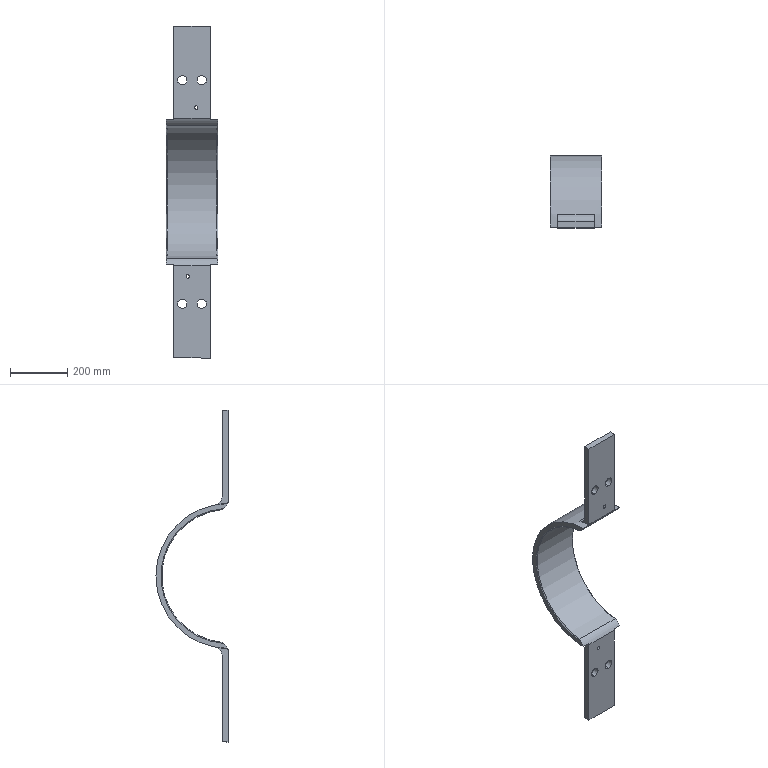Part | SolidWorks | features ICE 4, Fillet 2, MirrorPattern 2, Chamfer 1, Extrusion 1, HoleWzd 1 | 1 solid | 32 faces | box 180 x 251.8 x 1160 mm | volume 4341383 mm3 | cylinder 18 | plane 12 | cone 2 | commonest cylinder face diameters 32 x8 12 x4 60 x2 110 x2 466 x1 506 x1
STEP:
#1=CARTESIAN_POINT('',(-34.,22.,406.));
#2=VERTEX_POINT('',#1);
#3=CARTESIAN_POINT('',(-34.,22.,374.));
#4=VERTEX_POINT('',#3);
#5=CARTESIAN_POINT('',(-34.,22.,390.));
#6=DIRECTION('',(0.,-1.,0.));
#7=DIRECTION('',(0.,0.,-1.));
#8=AXIS2_PLACEMENT_3D('',#5,#6,#7);
#9=CIRCLE('',#8,16.);
#10=EDGE_CURVE('',#2,#4,#9,.T.);
#11=ORIENTED_EDGE('',*,*,#10,.F.);
#12=CARTESIAN_POINT('',(-34.,1.2,406.));
#13=VERTEX_POINT('',#12);
#14=CARTESIAN_POINT('',(-34.,1.2,406.));
#15=DIRECTION('',(0.,-1.,0.));
#16=VECTOR('',#15,1000.);
#17=LINE('',#14,#16);
#18=EDGE_CURVE('',#2,#13,#17,.T.);
#19=ORIENTED_EDGE('',*,*,#18,.T.);
#20=CARTESIAN_POINT('',(-34.,1.2,374.));
#21=VERTEX_POINT('',#20);
#22=CARTESIAN_POINT('',(-34.,1.2,390.));
#23=DIRECTION('',(0.,-1.,0.));
#24=DIRECTION('',(0.,0.,-1.));
#25=AXIS2_PLACEMENT_3D('',#22,#23,#24);
#26=CIRCLE('',#25,16.);
#27=EDGE_CURVE('',#13,#21,#26,.T.);
#28=ORIENTED_EDGE('',*,*,#27,.T.);
#29=CARTESIAN_POINT('',(-34.,1.2,374.));
#30=DIRECTION('',(0.,-1.,0.));
#31=VECTOR('',#30,1000.);
#32=LINE('',#29,#31);
#33=EDGE_CURVE('',#4,#21,#32,.T.);
#34=ORIENTED_EDGE('',*,*,#33,.F.);
#35=EDGE_LOOP('',(#11,#19,#28,#34));
#36=FACE_OUTER_BOUND('',#35,.T.);
#37=CARTESIAN_POINT('',(-34.,1.2,390.));
#38=DIRECTION('',(0.,-1.,0.));
#39=DIRECTION('',(0.,0.,-1.));
#40=AXIS2_PLACEMENT_3D('',#37,#38,#39);
#41=CYLINDRICAL_SURFACE('',#40,16.);
#42=ADVANCED_FACE('',(#36),#41,.F.);
#43=CARTESIAN_POINT('',(34.,22.,406.));
#44=VERTEX_POINT('',#43);
#45=CARTESIAN_POINT('',(34.,22.,374.));
#46=VERTEX_POINT('',#45);
#47=CARTESIAN_POINT('',(34.,22.,390.));
#48=DIRECTION('',(0.,-1.,0.));
#49=DIRECTION('',(0.,0.,-1.));
#50=AXIS2_PLACEMENT_3D('',#47,#48,#49);
#51=CIRCLE('',#50,16.);
#52=EDGE_CURVE('',#44,#46,#51,.T.);
#53=ORIENTED_EDGE('',*,*,#52,.F.);
#54=CARTESIAN_POINT('',(34.,1.2,406.));
#55=VERTEX_POINT('',#54);
#56=CARTESIAN_POINT('',(34.,1.2,406.));
#57=DIRECTION('',(0.,-1.,0.));
#58=VECTOR('',#57,1000.);
#59=LINE('',#56,#58);
#60=EDGE_CURVE('',#44,#55,#59,.T.);
#61=ORIENTED_EDGE('',*,*,#60,.T.);
#62=CARTESIAN_POINT('',(34.,1.2,374.));
#63=VERTEX_POINT('',#62);
#64=CARTESIAN_POINT('',(34.,1.2,390.));
#65=DIRECTION('',(0.,-1.,0.));
#66=DIRECTION('',(0.,0.,-1.));
#67=AXIS2_PLACEMENT_3D('',#64,#65,#66);
#68=CIRCLE('',#67,16.);
#69=EDGE_CURVE('',#55,#63,#68,.T.);
#70=ORIENTED_EDGE('',*,*,#69,.T.);
#71=CARTESIAN_POINT('',(34.,1.2,374.));
#72=DIRECTION('',(0.,-1.,0.));
#73=VECTOR('',#72,1000.);
#74=LINE('',#71,#73);
#75=EDGE_CURVE('',#46,#63,#74,.T.);
#76=ORIENTED_EDGE('',*,*,#75,.F.);
#77=EDGE_LOOP('',(#53,#61,#70,#76));
#78=FACE_OUTER_BOUND('',#77,.T.);
#79=CARTESIAN_POINT('',(34.,1.2,390.));
#80=DIRECTION('',(0.,-1.,0.));
#81=DIRECTION('',(0.,0.,-1.));
#82=AXIS2_PLACEMENT_3D('',#79,#80,#81);
#83=CYLINDRICAL_SURFACE('',#82,16.);
#84=ADVANCED_FACE('',(#78),#83,.F.);
#85=CARTESIAN_POINT('',(34.,22.,-374.));
#86=VERTEX_POINT('',#85);
#87=CARTESIAN_POINT('',(34.,22.,-406.));
#88=VERTEX_POINT('',#87);
#89=CARTESIAN_POINT('',(34.,22.,-390.));
#90=DIRECTION('',(0.,-1.,0.));
#91=DIRECTION('',(0.,0.,-1.));
#92=AXIS2_PLACEMENT_3D('',#89,#90,#91);
#93=CIRCLE('',#92,16.);
#94=EDGE_CURVE('',#86,#88,#93,.T.);
#95=ORIENTED_EDGE('',*,*,#94,.F.);
#96=CARTESIAN_POINT('',(34.,1.2,-374.));
#97=VERTEX_POINT('',#96);
#98=CARTESIAN_POINT('',(34.,1.2,-374.));
#99=DIRECTION('',(0.,-1.,0.));
#100=VECTOR('',#99,1000.);
#101=LINE('',#98,#100);
#102=EDGE_CURVE('',#86,#97,#101,.T.);
#103=ORIENTED_EDGE('',*,*,#102,.T.);
#104=CARTESIAN_POINT('',(34.,1.2,-406.));
#105=VERTEX_POINT('',#104);
#106=CARTESIAN_POINT('',(34.,1.2,-390.));
#107=DIRECTION('',(0.,-1.,0.));
#108=DIRECTION('',(0.,0.,-1.));
#109=AXIS2_PLACEMENT_3D('',#106,#107,#108);
#110=CIRCLE('',#109,16.);
#111=EDGE_CURVE('',#97,#105,#110,.T.);
#112=ORIENTED_EDGE('',*,*,#111,.T.);
#113=CARTESIAN_POINT('',(34.,1.2,-406.));
#114=DIRECTION('',(0.,-1.,0.));
#115=VECTOR('',#114,1000.);
#116=LINE('',#113,#115);
#117=EDGE_CURVE('',#88,#105,#116,.T.);
#118=ORIENTED_EDGE('',*,*,#117,.F.);
#119=EDGE_LOOP('',(#95,#103,#112,#118));
#120=FACE_OUTER_BOUND('',#119,.T.);
#121=CARTESIAN_POINT('',(34.,1.2,-390.));
#122=DIRECTION('',(0.,-1.,0.));
#123=DIRECTION('',(0.,0.,-1.));
#124=AXIS2_PLACEMENT_3D('',#121,#122,#123);
#125=CYLINDRICAL_SURFACE('',#124,16.);
#126=ADVANCED_FACE('',(#120),#125,.F.);
#127=CARTESIAN_POINT('',(-34.,22.,-374.));
#128=VERTEX_POINT('',#127);
#129=CARTESIAN_POINT('',(-34.,22.,-406.));
#130=VERTEX_POINT('',#129);
#131=CARTESIAN_POINT('',(-34.,22.,-390.));
#132=DIRECTION('',(0.,-1.,0.));
#133=DIRECTION('',(0.,0.,-1.));
#134=AXIS2_PLACEMENT_3D('',#131,#132,#133);
#135=CIRCLE('',#134,16.);
#136=EDGE_CURVE('',#128,#130,#135,.T.);
#137=ORIENTED_EDGE('',*,*,#136,.F.);
#138=CARTESIAN_POINT('',(-34.,1.2,-374.));
#139=VERTEX_POINT('',#138);
#140=CARTESIAN_POINT('',(-34.,1.2,-374.));
#141=DIRECTION('',(0.,-1.,0.));
#142=VECTOR('',#141,1000.);
#143=LINE('',#140,#142);
#144=EDGE_CURVE('',#128,#139,#143,.T.);
#145=ORIENTED_EDGE('',*,*,#144,.T.);
#146=CARTESIAN_POINT('',(-34.,1.2,-406.));
#147=VERTEX_POINT('',#146);
#148=CARTESIAN_POINT('',(-34.,1.2,-390.));
#149=DIRECTION('',(0.,-1.,0.));
#150=DIRECTION('',(0.,0.,-1.));
#151=AXIS2_PLACEMENT_3D('',#148,#149,#150);
#152=CIRCLE('',#151,16.);
#153=EDGE_CURVE('',#139,#147,#152,.T.);
#154=ORIENTED_EDGE('',*,*,#153,.T.);
#155=CARTESIAN_POINT('',(-34.,1.2,-406.));
#156=DIRECTION('',(0.,-1.,0.));
#157=VECTOR('',#156,1000.);
#158=LINE('',#155,#157);
#159=EDGE_CURVE('',#130,#147,#158,.T.);
#160=ORIENTED_EDGE('',*,*,#159,.F.);
#161=EDGE_LOOP('',(#137,#145,#154,#160));
#162=FACE_OUTER_BOUND('',#161,.T.);
#163=CARTESIAN_POINT('',(-34.,1.2,-390.));
#164=DIRECTION('',(0.,-1.,0.));
#165=DIRECTION('',(0.,0.,-1.));
#166=AXIS2_PLACEMENT_3D('',#163,#164,#165);
#167=CYLINDRICAL_SURFACE('',#166,16.);
#168=ADVANCED_FACE('',(#162),#167,.F.);
#169=CARTESIAN_POINT('',(-15.,22.,-301.));
#170=VERTEX_POINT('',#169);
#171=CARTESIAN_POINT('',(-15.,22.,-289.));
#172=VERTEX_POINT('',#171);
#173=CARTESIAN_POINT('',(-15.,22.,-295.));
#174=DIRECTION('',(0.,1.,0.));
#175=DIRECTION('',(0.,0.,-1.));
#176=AXIS2_PLACEMENT_3D('',#173,#174,#175);
#177=CIRCLE('',#176,6.);
#178=EDGE_CURVE('',#170,#172,#177,.T.);
#179=ORIENTED_EDGE('',*,*,#178,.T.);
#180=CARTESIAN_POINT('',(-15.,1.2,-289.));
#181=VERTEX_POINT('',#180);
#182=CARTESIAN_POINT('',(-15.,1.2,-289.));
#183=DIRECTION('',(0.,-1.,0.));
#184=VECTOR('',#183,1000.);
#185=LINE('',#182,#184);
#186=EDGE_CURVE('',#172,#181,#185,.T.);
#187=ORIENTED_EDGE('',*,*,#186,.T.);
#188=CARTESIAN_POINT('',(-15.,1.2,-301.));
#189=VERTEX_POINT('',#188);
#190=CARTESIAN_POINT('',(-15.,1.2,-295.));
#191=DIRECTION('',(0.,-1.,0.));
#192=DIRECTION('',(0.,0.,1.));
#193=AXIS2_PLACEMENT_3D('',#190,#191,#192);
#194=CIRCLE('',#193,6.);
#195=EDGE_CURVE('',#181,#189,#194,.T.);
#196=ORIENTED_EDGE('',*,*,#195,.T.);
#197=CARTESIAN_POINT('',(-15.,1.2,-301.));
#198=DIRECTION('',(0.,-1.,0.));
#199=VECTOR('',#198,1000.);
#200=LINE('',#197,#199);
#201=EDGE_CURVE('',#170,#189,#200,.T.);
#202=ORIENTED_EDGE('',*,*,#201,.F.);
#203=EDGE_LOOP('',(#179,#187,#196,#202));
#204=FACE_OUTER_BOUND('',#203,.T.);
#205=CARTESIAN_POINT('',(-15.,1.2,-295.));
#206=DIRECTION('',(0.,-1.,0.));
#207=DIRECTION('',(0.,0.,-1.));
#208=AXIS2_PLACEMENT_3D('',#205,#206,#207);
#209=CYLINDRICAL_SURFACE('',#208,6.);
#210=ADVANCED_FACE('',(#204),#209,.F.);
#211=CARTESIAN_POINT('',(15.,22.,289.));
#212=VERTEX_POINT('',#211);
#213=CARTESIAN_POINT('',(15.,22.,301.));
#214=VERTEX_POINT('',#213);
#215=CARTESIAN_POINT('',(15.,22.,295.));
#216=DIRECTION('',(0.,1.,0.));
#217=DIRECTION('',(0.,0.,-1.));
#218=AXIS2_PLACEMENT_3D('',#215,#216,#217);
#219=CIRCLE('',#218,6.);
#220=EDGE_CURVE('',#212,#214,#219,.T.);
#221=ORIENTED_EDGE('',*,*,#220,.T.);
#222=CARTESIAN_POINT('',(15.,1.2,301.));
#223=VERTEX_POINT('',#222);
#224=CARTESIAN_POINT('',(15.,1.2,301.));
#225=DIRECTION('',(0.,-1.,0.));
#226=VECTOR('',#225,1000.);
#227=LINE('',#224,#226);
#228=EDGE_CURVE('',#214,#223,#227,.T.);
#229=ORIENTED_EDGE('',*,*,#228,.T.);
#230=CARTESIAN_POINT('',(15.,1.2,289.));
#231=VERTEX_POINT('',#230);
#232=CARTESIAN_POINT('',(15.,1.2,295.));
#233=DIRECTION('',(0.,-1.,0.));
#234=DIRECTION('',(0.,0.,1.));
#235=AXIS2_PLACEMENT_3D('',#232,#233,#234);
#236=CIRCLE('',#235,6.);
#237=EDGE_CURVE('',#223,#231,#236,.T.);
#238=ORIENTED_EDGE('',*,*,#237,.T.);
#239=CARTESIAN_POINT('',(15.,1.2,289.));
#240=DIRECTION('',(0.,-1.,0.));
#241=VECTOR('',#240,1000.);
#242=LINE('',#239,#241);
#243=EDGE_CURVE('',#212,#231,#242,.T.);
#244=ORIENTED_EDGE('',*,*,#243,.F.);
#245=EDGE_LOOP('',(#221,#229,#238,#244));
#246=FACE_OUTER_BOUND('',#245,.T.);
#247=CARTESIAN_POINT('',(15.,1.2,295.));
#248=DIRECTION('',(0.,-1.,0.));
#249=DIRECTION('',(0.,0.,-1.));
#250=AXIS2_PLACEMENT_3D('',#247,#248,#249);
#251=CYLINDRICAL_SURFACE('',#250,6.);
#252=ADVANCED_FACE('',(#246),#251,.F.);
#253=CARTESIAN_POINT('',(34.,22.,-390.));
#254=DIRECTION('',(0.,-1.,0.));
#255=DIRECTION('',(0.,0.,-1.));
#256=AXIS2_PLACEMENT_3D('',#253,#254,#255);
#257=CIRCLE('',#256,16.);
#258=EDGE_CURVE('',#88,#86,#257,.T.);
#259=ORIENTED_EDGE('',*,*,#258,.T.);
#260=ORIENTED_EDGE('',*,*,#94,.T.);
#261=EDGE_LOOP('',(#259,#260));
#262=FACE_BOUND('',#261,.T.);
#263=CARTESIAN_POINT('',(-34.,22.,-390.));
#264=DIRECTION('',(0.,-1.,0.));
#265=DIRECTION('',(0.,0.,-1.));
#266=AXIS2_PLACEMENT_3D('',#263,#264,#265);
#267=CIRCLE('',#266,16.);
#268=EDGE_CURVE('',#130,#128,#267,.T.);
#269=ORIENTED_EDGE('',*,*,#268,.T.);
#270=ORIENTED_EDGE('',*,*,#136,.T.);
#271=EDGE_LOOP('',(#269,#270));
#272=FACE_BOUND('',#271,.T.);
#273=CARTESIAN_POINT('',(-63.,22.,-278.182));
#274=VERTEX_POINT('',#273);
#275=CARTESIAN_POINT('',(-63.,22.,-580.));
#276=VERTEX_POINT('',#275);
#277=CARTESIAN_POINT('',(-63.,22.,-252.042));
#278=DIRECTION('',(0.,0.,-1.));
#279=VECTOR('',#278,1000.);
#280=LINE('',#277,#279);
#281=EDGE_CURVE('',#274,#276,#280,.T.);
#282=ORIENTED_EDGE('',*,*,#281,.F.);
#283=CARTESIAN_POINT('',(63.,22.,-278.182));
#284=VERTEX_POINT('',#283);
#285=CARTESIAN_POINT('',(90.,22.,-278.182));
#286=DIRECTION('',(1.,0.,0.));
#287=VECTOR('',#286,1000.);
#288=LINE('',#285,#287);
#289=EDGE_CURVE('',#274,#284,#288,.T.);
#290=ORIENTED_EDGE('',*,*,#289,.T.);
#291=CARTESIAN_POINT('',(63.,22.,-580.));
#292=VERTEX_POINT('',#291);
#293=CARTESIAN_POINT('',(63.,22.,-252.042));
#294=DIRECTION('',(0.,0.,1.));
#295=VECTOR('',#294,1000.);
#296=LINE('',#293,#295);
#297=EDGE_CURVE('',#292,#284,#296,.T.);
#298=ORIENTED_EDGE('',*,*,#297,.F.);
#299=CARTESIAN_POINT('',(90.,22.,-580.));
#300=DIRECTION('',(-1.,0.,0.));
#301=VECTOR('',#300,1000.);
#302=LINE('',#299,#301);
#303=EDGE_CURVE('',#292,#276,#302,.T.);
#304=ORIENTED_EDGE('',*,*,#303,.T.);
#305=EDGE_LOOP('',(#282,#290,#298,#304));
#306=FACE_OUTER_BOUND('',#305,.T.);
#307=ORIENTED_EDGE('',*,*,#178,.F.);
#308=CARTESIAN_POINT('',(-15.,22.,-295.));
#309=DIRECTION('',(0.,1.,0.));
#310=DIRECTION('',(0.,0.,-1.));
#311=AXIS2_PLACEMENT_3D('',#308,#309,#310);
#312=CIRCLE('',#311,6.);
#313=EDGE_CURVE('',#172,#170,#312,.T.);
#314=ORIENTED_EDGE('',*,*,#313,.F.);
#315=EDGE_LOOP('',(#307,#314));
#316=FACE_BOUND('',#315,.T.);
#317=CARTESIAN_POINT('',(90.,22.,-252.042));
#318=DIRECTION('',(0.,-1.,0.));
#319=DIRECTION('',(0.,0.,-1.));
#320=AXIS2_PLACEMENT_3D('',#317,#318,#319);
#321=PLANE('',#320);
#322=ADVANCED_FACE('',(#262,#272,#306,#316),#321,.F.);
#323=CARTESIAN_POINT('',(34.,1.2,-390.));
#324=DIRECTION('',(0.,-1.,0.));
#325=DIRECTION('',(0.,0.,-1.));
#326=AXIS2_PLACEMENT_3D('',#323,#324,#325);
#327=CIRCLE('',#326,16.);
#328=EDGE_CURVE('',#105,#97,#327,.T.);
#329=ORIENTED_EDGE('',*,*,#328,.F.);
#330=ORIENTED_EDGE('',*,*,#111,.F.);
#331=EDGE_LOOP('',(#329,#330));
#332=FACE_BOUND('',#331,.T.);
#333=CARTESIAN_POINT('',(-34.,1.2,-390.));
#334=DIRECTION('',(0.,-1.,0.));
#335=DIRECTION('',(0.,0.,-1.));
#336=AXIS2_PLACEMENT_3D('',#333,#334,#335);
#337=CIRCLE('',#336,16.);
#338=EDGE_CURVE('',#147,#139,#337,.T.);
#339=ORIENTED_EDGE('',*,*,#338,.F.);
#340=ORIENTED_EDGE('',*,*,#153,.F.);
#341=EDGE_LOOP('',(#339,#340));
#342=FACE_BOUND('',#341,.T.);
#343=CARTESIAN_POINT('',(-63.,1.2,-580.));
#344=VERTEX_POINT('',#343);
#345=CARTESIAN_POINT('',(-63.,1.2,-257.102));
#346=VERTEX_POINT('',#345);
#347=CARTESIAN_POINT('',(-63.,1.2,610.));
#348=DIRECTION('',(0.,0.,1.));
#349=VECTOR('',#348,1000.);
#350=LINE('',#347,#349);
#351=EDGE_CURVE('',#344,#346,#350,.T.);
#352=ORIENTED_EDGE('',*,*,#351,.F.);
#353=CARTESIAN_POINT('',(63.,1.2,-580.));
#354=VERTEX_POINT('',#353);
#355=CARTESIAN_POINT('',(90.,1.2,-580.));
#356=DIRECTION('',(-1.,0.,0.));
#357=VECTOR('',#356,1000.);
#358=LINE('',#355,#357);
#359=EDGE_CURVE('',#354,#344,#358,.T.);
#360=ORIENTED_EDGE('',*,*,#359,.F.);
#361=CARTESIAN_POINT('',(63.,1.2,-257.102));
#362=VERTEX_POINT('',#361);
#363=CARTESIAN_POINT('',(63.,1.2,610.));
#364=DIRECTION('',(0.,0.,-1.));
#365=VECTOR('',#364,1000.);
#366=LINE('',#363,#365);
#367=EDGE_CURVE('',#362,#354,#366,.T.);
#368=ORIENTED_EDGE('',*,*,#367,.F.);
#369=CARTESIAN_POINT('',(90.,1.2,-257.102));
#370=DIRECTION('',(-1.,0.,0.));
#371=VECTOR('',#370,1000.);
#372=LINE('',#369,#371);
#373=EDGE_CURVE('',#362,#346,#372,.T.);
#374=ORIENTED_EDGE('',*,*,#373,.T.);
#375=EDGE_LOOP('',(#352,#360,#368,#374));
#376=FACE_OUTER_BOUND('',#375,.T.);
#377=CARTESIAN_POINT('',(-15.,1.2,-295.));
#378=DIRECTION('',(0.,-1.,0.));
#379=DIRECTION('',(0.,0.,1.));
#380=AXIS2_PLACEMENT_3D('',#377,#378,#379);
#381=CIRCLE('',#380,6.);
#382=EDGE_CURVE('',#189,#181,#381,.T.);
#383=ORIENTED_EDGE('',*,*,#382,.F.);
#384=ORIENTED_EDGE('',*,*,#195,.F.);
#385=EDGE_LOOP('',(#383,#384));
#386=FACE_BOUND('',#385,.T.);
#387=CARTESIAN_POINT('',(-90.,1.2,610.));
#388=DIRECTION('',(0.,1.,0.));
#389=DIRECTION('',(0.,0.,1.));
#390=AXIS2_PLACEMENT_3D('',#387,#388,#389);
#391=PLANE('',#390);
#392=ADVANCED_FACE('',(#332,#342,#376,#386),#391,.F.);
#393=CARTESIAN_POINT('',(-34.,22.,390.));
#394=DIRECTION('',(0.,-1.,0.));
#395=DIRECTION('',(0.,0.,-1.));
#396=AXIS2_PLACEMENT_3D('',#393,#394,#395);
#397=CIRCLE('',#396,16.);
#398=EDGE_CURVE('',#4,#2,#397,.T.);
#399=ORIENTED_EDGE('',*,*,#398,.T.);
#400=ORIENTED_EDGE('',*,*,#10,.T.);
#401=EDGE_LOOP('',(#399,#400));
#402=FACE_BOUND('',#401,.T.);
#403=CARTESIAN_POINT('',(34.,22.,390.));
#404=DIRECTION('',(0.,-1.,0.));
#405=DIRECTION('',(0.,0.,-1.));
#406=AXIS2_PLACEMENT_3D('',#403,#404,#405);
#407=CIRCLE('',#406,16.);
#408=EDGE_CURVE('',#46,#44,#407,.T.);
#409=ORIENTED_EDGE('',*,*,#408,.T.);
#410=ORIENTED_EDGE('',*,*,#52,.T.);
#411=EDGE_LOOP('',(#409,#410));
#412=FACE_BOUND('',#411,.T.);
#413=CARTESIAN_POINT('',(-63.,22.,580.));
#414=VERTEX_POINT('',#413);
#415=CARTESIAN_POINT('',(-63.,22.,278.182));
#416=VERTEX_POINT('',#415);
#417=CARTESIAN_POINT('',(-63.,22.,580.));
#418=DIRECTION('',(0.,0.,-1.));
#419=VECTOR('',#418,1000.);
#420=LINE('',#417,#419);
#421=EDGE_CURVE('',#414,#416,#420,.T.);
#422=ORIENTED_EDGE('',*,*,#421,.F.);
#423=CARTESIAN_POINT('',(63.,22.,580.));
#424=VERTEX_POINT('',#423);
#425=CARTESIAN_POINT('',(90.,22.,580.));
#426=DIRECTION('',(-1.,0.,0.));
#427=VECTOR('',#426,1000.);
#428=LINE('',#425,#427);
#429=EDGE_CURVE('',#424,#414,#428,.T.);
#430=ORIENTED_EDGE('',*,*,#429,.F.);
#431=CARTESIAN_POINT('',(63.,22.,278.182));
#432=VERTEX_POINT('',#431);
#433=CARTESIAN_POINT('',(63.,22.,580.));
#434=DIRECTION('',(0.,0.,1.));
#435=VECTOR('',#434,1000.);
#436=LINE('',#433,#435);
#437=EDGE_CURVE('',#432,#424,#436,.T.);
#438=ORIENTED_EDGE('',*,*,#437,.F.);
#439=CARTESIAN_POINT('',(-90.,22.,278.182));
#440=DIRECTION('',(-1.,0.,0.));
#441=VECTOR('',#440,1000.);
#442=LINE('',#439,#441);
#443=EDGE_CURVE('',#432,#416,#442,.T.);
#444=ORIENTED_EDGE('',*,*,#443,.T.);
#445=EDGE_LOOP('',(#422,#430,#438,#444));
#446=FACE_OUTER_BOUND('',#445,.T.);
#447=ORIENTED_EDGE('',*,*,#220,.F.);
#448=CARTESIAN_POINT('',(15.,22.,295.));
#449=DIRECTION('',(0.,1.,0.));
#450=DIRECTION('',(0.,0.,-1.));
#451=AXIS2_PLACEMENT_3D('',#448,#449,#450);
#452=CIRCLE('',#451,6.);
#453=EDGE_CURVE('',#214,#212,#452,.T.);
#454=ORIENTED_EDGE('',*,*,#453,.F.);
#455=EDGE_LOOP('',(#447,#454));
#456=FACE_BOUND('',#455,.T.);
#457=CARTESIAN_POINT('',(90.,22.,580.));
#458=DIRECTION('',(0.,-1.,0.));
#459=DIRECTION('',(0.,0.,-1.));
#460=AXIS2_PLACEMENT_3D('',#457,#458,#459);
#461=PLANE('',#460);
#462=ADVANCED_FACE('',(#402,#412,#446,#456),#461,.F.);
#463=CARTESIAN_POINT('',(-34.,1.2,390.));
#464=DIRECTION('',(0.,-1.,0.));
#465=DIRECTION('',(0.,0.,-1.));
#466=AXIS2_PLACEMENT_3D('',#463,#464,#465);
#467=CIRCLE('',#466,16.);
#468=EDGE_CURVE('',#21,#13,#467,.T.);
#469=ORIENTED_EDGE('',*,*,#468,.F.);
#470=ORIENTED_EDGE('',*,*,#27,.F.);
#471=EDGE_LOOP('',(#469,#470));
#472=FACE_BOUND('',#471,.T.);
#473=CARTESIAN_POINT('',(34.,1.2,390.));
#474=DIRECTION('',(0.,-1.,0.));
#475=DIRECTION('',(0.,0.,-1.));
#476=AXIS2_PLACEMENT_3D('',#473,#474,#475);
#477=CIRCLE('',#476,16.);
#478=EDGE_CURVE('',#63,#55,#477,.T.);
#479=ORIENTED_EDGE('',*,*,#478,.F.);
#480=ORIENTED_EDGE('',*,*,#69,.F.);
#481=EDGE_LOOP('',(#479,#480));
#482=FACE_BOUND('',#481,.T.);
#483=CARTESIAN_POINT('',(-63.,1.2,257.102));
#484=VERTEX_POINT('',#483);
#485=CARTESIAN_POINT('',(-63.,1.2,580.));
#486=VERTEX_POINT('',#485);
#487=CARTESIAN_POINT('',(-63.,1.2,610.));
#488=DIRECTION('',(0.,0.,1.));
#489=VECTOR('',#488,1000.);
#490=LINE('',#487,#489);
#491=EDGE_CURVE('',#484,#486,#490,.T.);
#492=ORIENTED_EDGE('',*,*,#491,.F.);
#493=CARTESIAN_POINT('',(63.,1.2,257.102));
#494=VERTEX_POINT('',#493);
#495=CARTESIAN_POINT('',(90.,1.2,257.102));
#496=DIRECTION('',(1.,0.,0.));
#497=VECTOR('',#496,1000.);
#498=LINE('',#495,#497);
#499=EDGE_CURVE('',#484,#494,#498,.T.);
#500=ORIENTED_EDGE('',*,*,#499,.T.);
#501=CARTESIAN_POINT('',(63.,1.2,580.));
#502=VERTEX_POINT('',#501);
#503=CARTESIAN_POINT('',(63.,1.2,610.));
#504=DIRECTION('',(0.,0.,-1.));
#505=VECTOR('',#504,1000.);
#506=LINE('',#503,#505);
#507=EDGE_CURVE('',#502,#494,#506,.T.);
#508=ORIENTED_EDGE('',*,*,#507,.F.);
#509=CARTESIAN_POINT('',(90.,1.2,580.));
#510=DIRECTION('',(1.,0.,0.));
#511=VECTOR('',#510,1000.);
#512=LINE('',#509,#511);
#513=EDGE_CURVE('',#486,#502,#512,.T.);
#514=ORIENTED_EDGE('',*,*,#513,.F.);
#515=EDGE_LOOP('',(#492,#500,#508,#514));
#516=FACE_OUTER_BOUND('',#515,.T.);
#517=CARTESIAN_POINT('',(15.,1.2,295.));
#518=DIRECTION('',(0.,-1.,0.));
#519=DIRECTION('',(0.,0.,1.));
#520=AXIS2_PLACEMENT_3D('',#517,#518,#519);
#521=CIRCLE('',#520,6.);
#522=EDGE_CURVE('',#231,#223,#521,.T.);
#523=ORIENTED_EDGE('',*,*,#522,.F.);
#524=ORIENTED_EDGE('',*,*,#237,.F.);
#525=EDGE_LOOP('',(#523,#524));
#526=FACE_BOUND('',#525,.T.);
#527=CARTESIAN_POINT('',(-90.,1.2,610.));
#528=DIRECTION('',(0.,1.,0.));
#529=DIRECTION('',(0.,0.,1.));
#530=AXIS2_PLACEMENT_3D('',#527,#528,#529);
#531=PLANE('',#530);
#532=ADVANCED_FACE('',(#472,#482,#516,#526),#531,.F.);
#533=CARTESIAN_POINT('',(-63.,22.,-580.));
#534=DIRECTION('',(0.,-1.,0.));
#535=VECTOR('',#534,1000.);
#536=LINE('',#533,#535);
#537=EDGE_CURVE('',#276,#344,#536,.T.);
#538=ORIENTED_EDGE('',*,*,#537,.F.);
#539=ORIENTED_EDGE('',*,*,#303,.F.);
#540=CARTESIAN_POINT('',(63.,22.,-580.));
#541=DIRECTION('',(0.,1.,0.));
#542=VECTOR('',#541,1000.);
#543=LINE('',#540,#542);
#544=EDGE_CURVE('',#354,#292,#543,.T.);
#545=ORIENTED_EDGE('',*,*,#544,.F.);
#546=ORIENTED_EDGE('',*,*,#359,.T.);
#547=EDGE_LOOP('',(#538,#539,#545,#546));
#548=FACE_OUTER_BOUND('',#547,.T.);
#549=CARTESIAN_POINT('',(90.,22.,-580.));
#550=DIRECTION('',(0.,0.,1.));
#551=DIRECTION('',(1.,0.,0.));
#552=AXIS2_PLACEMENT_3D('',#549,#550,#551);
#553=PLANE('',#552);
#554=ADVANCED_FACE('',(#548),#553,.F.);
#555=CARTESIAN_POINT('',(-63.,46.488,-248.692));
#556=VERTEX_POINT('',#555);
#557=CARTESIAN_POINT('',(-63.,52.,-278.182));
#558=DIRECTION('',(1.,0.,0.));
#559=DIRECTION('',(0.,0.,1.));
#560=AXIS2_PLACEMENT_3D('',#557,#558,#559);
#561=CIRCLE('',#560,30.);
#562=EDGE_CURVE('',#556,#274,#561,.T.);
#563=ORIENTED_EDGE('',*,*,#562,.F.);
#564=CARTESIAN_POINT('',(63.,46.488,-248.692));
#565=VERTEX_POINT('',#564);
#566=CARTESIAN_POINT('',(90.,46.488,-248.692));
#567=DIRECTION('',(-1.,0.,0.));
#568=VECTOR('',#567,1000.);
#569=LINE('',#566,#568);
#570=EDGE_CURVE('',#565,#556,#569,.T.);
#571=ORIENTED_EDGE('',*,*,#570,.F.);
#572=CARTESIAN_POINT('',(63.,52.,-278.182));
#573=DIRECTION('',(-1.,0.,0.));
#574=DIRECTION('',(0.,0.,-1.));
#575=AXIS2_PLACEMENT_3D('',#572,#573,#574);
#576=CIRCLE('',#575,30.);
#577=EDGE_CURVE('',#284,#565,#576,.T.);
#578=ORIENTED_EDGE('',*,*,#577,.F.);
#579=ORIENTED_EDGE('',*,*,#289,.F.);
#580=EDGE_LOOP('',(#563,#571,#578,#579));
#581=FACE_OUTER_BOUND('',#580,.T.);
#582=CARTESIAN_POINT('',(90.,52.,-278.182));
#583=DIRECTION('',(-1.,0.,0.));
#584=DIRECTION('',(0.,0.,1.));
#585=AXIS2_PLACEMENT_3D('',#582,#583,#584);
#586=CYLINDRICAL_SURFACE('',#585,30.);
#587=ADVANCED_FACE('',(#581),#586,.F.);
#588=CARTESIAN_POINT('',(-63.,22.,580.));
#589=DIRECTION('',(0.,1.,0.));
#590=VECTOR('',#589,1000.);
#591=LINE('',#588,#590);
#592=EDGE_CURVE('',#486,#414,#591,.T.);
#593=ORIENTED_EDGE('',*,*,#592,.F.);
#594=ORIENTED_EDGE('',*,*,#513,.T.);
#595=CARTESIAN_POINT('',(63.,22.,580.));
#596=DIRECTION('',(0.,-1.,0.));
#597=VECTOR('',#596,1000.);
#598=LINE('',#595,#597);
#599=EDGE_CURVE('',#424,#502,#598,.T.);
#600=ORIENTED_EDGE('',*,*,#599,.F.);
#601=ORIENTED_EDGE('',*,*,#429,.T.);
#602=EDGE_LOOP('',(#593,#594,#600,#601));
#603=FACE_OUTER_BOUND('',#602,.T.);
#604=CARTESIAN_POINT('',(90.,22.,580.));
#605=DIRECTION('',(0.,0.,-1.));
#606=DIRECTION('',(-1.,0.,0.));
#607=AXIS2_PLACEMENT_3D('',#604,#605,#606);
#608=PLANE('',#607);
#609=ADVANCED_FACE('',(#603),#608,.F.);
#610=CARTESIAN_POINT('',(-63.,46.488,248.692));
#611=VERTEX_POINT('',#610);
#612=CARTESIAN_POINT('',(-63.,52.,278.182));
#613=DIRECTION('',(1.,0.,0.));
#614=DIRECTION('',(0.,0.,1.));
#615=AXIS2_PLACEMENT_3D('',#612,#613,#614);
#616=CIRCLE('',#615,30.);
#617=EDGE_CURVE('',#416,#611,#616,.T.);
#618=ORIENTED_EDGE('',*,*,#617,.F.);
#619=ORIENTED_EDGE('',*,*,#443,.F.);
#620=CARTESIAN_POINT('',(63.,46.488,248.692));
#621=VERTEX_POINT('',#620);
#622=CARTESIAN_POINT('',(63.,52.,278.182));
#623=DIRECTION('',(-1.,0.,0.));
#624=DIRECTION('',(0.,0.,-1.));
#625=AXIS2_PLACEMENT_3D('',#622,#623,#624);
#626=CIRCLE('',#625,30.);
#627=EDGE_CURVE('',#621,#432,#626,.T.);
#628=ORIENTED_EDGE('',*,*,#627,.F.);
#629=CARTESIAN_POINT('',(90.,46.488,248.692));
#630=DIRECTION('',(1.,0.,0.));
#631=VECTOR('',#630,1000.);
#632=LINE('',#629,#631);
#633=EDGE_CURVE('',#611,#621,#632,.T.);
#634=ORIENTED_EDGE('',*,*,#633,.F.);
#635=EDGE_LOOP('',(#618,#619,#628,#634));
#636=FACE_OUTER_BOUND('',#635,.T.);
#637=CARTESIAN_POINT('',(90.,52.,278.182));
#638=DIRECTION('',(-1.,0.,0.));
#639=DIRECTION('',(0.,0.,1.));
#640=AXIS2_PLACEMENT_3D('',#637,#638,#639);
#641=CYLINDRICAL_SURFACE('',#640,30.);
#642=ADVANCED_FACE('',(#636),#641,.F.);
#643=CARTESIAN_POINT('',(-90.,3.113,-252.981));
#644=VERTEX_POINT('',#643);
#645=CARTESIAN_POINT('',(-90.,17.496,-235.351));
#646=VERTEX_POINT('',#645);
#647=CARTESIAN_POINT('',(-90.,52.,-278.182));
#648=DIRECTION('',(-1.,0.,0.));
#649=DIRECTION('',(0.,0.,-1.));
#650=AXIS2_PLACEMENT_3D('',#647,#648,#649);
#651=CIRCLE('',#650,55.);
#652=EDGE_CURVE('',#644,#646,#651,.T.);
#653=ORIENTED_EDGE('',*,*,#652,.T.);
#654=CARTESIAN_POINT('',(-90.,17.496,235.351));
#655=VERTEX_POINT('',#654);
#656=CARTESIAN_POINT('',(-90.,0.,0.));
#657=DIRECTION('',(1.,0.,0.));
#658=DIRECTION('',(0.,0.,-1.));
#659=AXIS2_PLACEMENT_3D('',#656,#657,#658);
#660=CIRCLE('',#659,236.);
#661=EDGE_CURVE('',#646,#655,#660,.T.);
#662=ORIENTED_EDGE('',*,*,#661,.T.);
#663=CARTESIAN_POINT('',(-90.,3.113,252.981));
#664=VERTEX_POINT('',#663);
#665=CARTESIAN_POINT('',(-90.,52.,278.182));
#666=DIRECTION('',(-1.,0.,0.));
#667=DIRECTION('',(0.,0.,-1.));
#668=AXIS2_PLACEMENT_3D('',#665,#666,#667);
#669=CIRCLE('',#668,55.);
#670=EDGE_CURVE('',#655,#664,#669,.T.);
#671=ORIENTED_EDGE('',*,*,#670,.T.);
#672=CARTESIAN_POINT('',(-90.,0.,0.));
#673=DIRECTION('',(1.,0.,0.));
#674=DIRECTION('',(0.,0.,-1.));
#675=AXIS2_PLACEMENT_3D('',#672,#673,#674);
#676=CIRCLE('',#675,253.);
#677=EDGE_CURVE('',#644,#664,#676,.T.);
#678=ORIENTED_EDGE('',*,*,#677,.F.);
#679=EDGE_LOOP('',(#653,#662,#671,#678));
#680=FACE_OUTER_BOUND('',#679,.T.);
#681=CARTESIAN_POINT('',(-90.,0.,0.));
#682=DIRECTION('',(1.,0.,0.));
#683=DIRECTION('',(0.,0.,-1.));
#684=AXIS2_PLACEMENT_3D('',#681,#682,#683);
#685=PLANE('',#684);
#686=ADVANCED_FACE('',(#680),#685,.F.);
#687=CARTESIAN_POINT('',(87.,22.226,231.937));
#688=VERTEX_POINT('',#687);
#689=CARTESIAN_POINT('',(-87.,22.226,231.937));
#690=VERTEX_POINT('',#689);
#691=CARTESIAN_POINT('',(0.,22.226,231.937));
#692=DIRECTION('',(-1.,0.,0.));
#693=VECTOR('',#692,1000.);
#694=LINE('',#691,#693);
#695=EDGE_CURVE('',#688,#690,#694,.T.);
#696=ORIENTED_EDGE('',*,*,#695,.F.);
#697=CARTESIAN_POINT('',(90.,17.496,235.351));
#698=VERTEX_POINT('',#697);
#699=CARTESIAN_POINT('',(87.,22.226,231.937));
#700=CARTESIAN_POINT('',(87.913,20.552,233.016));
#701=CARTESIAN_POINT('',(88.918,18.98,234.156));
#702=CARTESIAN_POINT('',(90.,17.496,235.351));
#703=B_SPLINE_CURVE_WITH_KNOTS('',3,(#699,#700,#701,#702),.UNSPECIFIED.,.F.,.F.,(4,4),(0.,0.006559),.UNSPECIFIED.);
#704=EDGE_CURVE('',#688,#698,#703,.T.);
#705=ORIENTED_EDGE('',*,*,#704,.T.);
#706=CARTESIAN_POINT('',(90.,3.113,252.981));
#707=VERTEX_POINT('',#706);
#708=CARTESIAN_POINT('',(90.,52.,278.182));
#709=DIRECTION('',(1.,0.,0.));
#710=DIRECTION('',(0.,0.,-1.));
#711=AXIS2_PLACEMENT_3D('',#708,#709,#710);
#712=CIRCLE('',#711,55.);
#713=EDGE_CURVE('',#707,#698,#712,.T.);
#714=ORIENTED_EDGE('',*,*,#713,.F.);
#715=CARTESIAN_POINT('',(63.,3.113,252.981));
#716=VERTEX_POINT('',#715);
#717=CARTESIAN_POINT('',(76.5,3.113,252.981));
#718=DIRECTION('',(1.,0.,0.));
#719=VECTOR('',#718,1000.);
#720=LINE('',#717,#719);
#721=EDGE_CURVE('',#716,#707,#720,.T.);
#722=ORIENTED_EDGE('',*,*,#721,.F.);
#723=CARTESIAN_POINT('',(63.,52.,278.182));
#724=DIRECTION('',(-1.,0.,0.));
#725=DIRECTION('',(0.,0.,-1.));
#726=AXIS2_PLACEMENT_3D('',#723,#724,#725);
#727=CIRCLE('',#726,55.);
#728=EDGE_CURVE('',#716,#494,#727,.T.);
#729=ORIENTED_EDGE('',*,*,#728,.T.);
#730=ORIENTED_EDGE('',*,*,#499,.F.);
#731=CARTESIAN_POINT('',(-63.,3.113,252.981));
#732=VERTEX_POINT('',#731);
#733=CARTESIAN_POINT('',(-63.,52.,278.182));
#734=DIRECTION('',(1.,0.,0.));
#735=DIRECTION('',(0.,0.,1.));
#736=AXIS2_PLACEMENT_3D('',#733,#734,#735);
#737=CIRCLE('',#736,55.);
#738=EDGE_CURVE('',#484,#732,#737,.T.);
#739=ORIENTED_EDGE('',*,*,#738,.T.);
#740=CARTESIAN_POINT('',(-76.5,3.113,252.981));
#741=DIRECTION('',(-1.,0.,0.));
#742=VECTOR('',#741,1000.);
#743=LINE('',#740,#742);
#744=EDGE_CURVE('',#732,#664,#743,.T.);
#745=ORIENTED_EDGE('',*,*,#744,.T.);
#746=ORIENTED_EDGE('',*,*,#670,.F.);
#747=CARTESIAN_POINT('',(-90.,17.496,235.351));
#748=CARTESIAN_POINT('',(-88.918,18.98,234.156));
#749=CARTESIAN_POINT('',(-87.913,20.552,233.016));
#750=CARTESIAN_POINT('',(-87.,22.226,231.937));
#751=B_SPLINE_CURVE_WITH_KNOTS('',3,(#747,#748,#749,#750),.UNSPECIFIED.,.F.,.F.,(4,4),(0.,0.006559),.UNSPECIFIED.);
#752=EDGE_CURVE('',#655,#690,#751,.T.);
#753=ORIENTED_EDGE('',*,*,#752,.T.);
#754=EDGE_LOOP('',(#696,#705,#714,#722,#729,#730,#739,#745,#746,#753));
#755=FACE_OUTER_BOUND('',#754,.T.);
#756=CARTESIAN_POINT('',(90.,52.,278.182));
#757=DIRECTION('',(-1.,0.,0.));
#758=DIRECTION('',(0.,0.,1.));
#759=AXIS2_PLACEMENT_3D('',#756,#757,#758);
#760=CYLINDRICAL_SURFACE('',#759,55.);
#761=ADVANCED_FACE('',(#755),#760,.T.);
#762=ORIENTED_EDGE('',*,*,#713,.T.);
#763=CARTESIAN_POINT('',(90.,17.496,-235.351));
#764=VERTEX_POINT('',#763);
#765=CARTESIAN_POINT('',(90.,0.,0.));
#766=DIRECTION('',(-1.,0.,0.));
#767=DIRECTION('',(0.,0.,-1.));
#768=AXIS2_PLACEMENT_3D('',#765,#766,#767);
#769=CIRCLE('',#768,236.);
#770=EDGE_CURVE('',#698,#764,#769,.T.);
#771=ORIENTED_EDGE('',*,*,#770,.T.);
#772=CARTESIAN_POINT('',(90.,3.113,-252.981));
#773=VERTEX_POINT('',#772);
#774=CARTESIAN_POINT('',(90.,52.,-278.182));
#775=DIRECTION('',(1.,0.,0.));
#776=DIRECTION('',(0.,0.,-1.));
#777=AXIS2_PLACEMENT_3D('',#774,#775,#776);
#778=CIRCLE('',#777,55.);
#779=EDGE_CURVE('',#764,#773,#778,.T.);
#780=ORIENTED_EDGE('',*,*,#779,.T.);
#781=CARTESIAN_POINT('',(90.,0.,0.));
#782=DIRECTION('',(1.,0.,0.));
#783=DIRECTION('',(0.,0.,-1.));
#784=AXIS2_PLACEMENT_3D('',#781,#782,#783);
#785=CIRCLE('',#784,253.);
#786=EDGE_CURVE('',#773,#707,#785,.T.);
#787=ORIENTED_EDGE('',*,*,#786,.T.);
#788=EDGE_LOOP('',(#762,#771,#780,#787));
#789=FACE_OUTER_BOUND('',#788,.T.);
#790=CARTESIAN_POINT('',(90.,0.,0.));
#791=DIRECTION('',(1.,0.,0.));
#792=DIRECTION('',(0.,0.,-1.));
#793=AXIS2_PLACEMENT_3D('',#790,#791,#792);
#794=PLANE('',#793);
#795=ADVANCED_FACE('',(#789),#794,.T.);
#796=ORIENTED_EDGE('',*,*,#779,.F.);
#797=CARTESIAN_POINT('',(87.,22.226,-231.937));
#798=VERTEX_POINT('',#797);
#799=CARTESIAN_POINT('',(90.,17.496,-235.351));
#800=CARTESIAN_POINT('',(88.918,18.98,-234.156));
#801=CARTESIAN_POINT('',(87.913,20.552,-233.016));
#802=CARTESIAN_POINT('',(87.,22.226,-231.937));
#803=B_SPLINE_CURVE_WITH_KNOTS('',3,(#799,#800,#801,#802),.UNSPECIFIED.,.F.,.F.,(4,4),(0.,0.006559),.UNSPECIFIED.);
#804=EDGE_CURVE('',#764,#798,#803,.T.);
#805=ORIENTED_EDGE('',*,*,#804,.T.);
#806=CARTESIAN_POINT('',(-87.,22.226,-231.937));
#807=VERTEX_POINT('',#806);
#808=CARTESIAN_POINT('',(0.,22.226,-231.937));
#809=DIRECTION('',(1.,0.,0.));
#810=VECTOR('',#809,1000.);
#811=LINE('',#808,#810);
#812=EDGE_CURVE('',#807,#798,#811,.T.);
#813=ORIENTED_EDGE('',*,*,#812,.F.);
#814=CARTESIAN_POINT('',(-87.,22.226,-231.937));
#815=CARTESIAN_POINT('',(-87.913,20.552,-233.016));
#816=CARTESIAN_POINT('',(-88.918,18.98,-234.156));
#817=CARTESIAN_POINT('',(-90.,17.496,-235.351));
#818=B_SPLINE_CURVE_WITH_KNOTS('',3,(#814,#815,#816,#817),.UNSPECIFIED.,.F.,.F.,(4,4),(0.,0.006559),.UNSPECIFIED.);
#819=EDGE_CURVE('',#807,#646,#818,.T.);
#820=ORIENTED_EDGE('',*,*,#819,.T.);
#821=ORIENTED_EDGE('',*,*,#652,.F.);
#822=CARTESIAN_POINT('',(-63.,3.113,-252.981));
#823=VERTEX_POINT('',#822);
#824=CARTESIAN_POINT('',(-76.5,3.113,-252.981));
#825=DIRECTION('',(-1.,0.,0.));
#826=VECTOR('',#825,1000.);
#827=LINE('',#824,#826);
#828=EDGE_CURVE('',#823,#644,#827,.T.);
#829=ORIENTED_EDGE('',*,*,#828,.F.);
#830=CARTESIAN_POINT('',(-63.,52.,-278.182));
#831=DIRECTION('',(1.,0.,0.));
#832=DIRECTION('',(0.,0.,1.));
#833=AXIS2_PLACEMENT_3D('',#830,#831,#832);
#834=CIRCLE('',#833,55.);
#835=EDGE_CURVE('',#823,#346,#834,.T.);
#836=ORIENTED_EDGE('',*,*,#835,.T.);
#837=ORIENTED_EDGE('',*,*,#373,.F.);
#838=CARTESIAN_POINT('',(63.,3.113,-252.981));
#839=VERTEX_POINT('',#838);
#840=CARTESIAN_POINT('',(63.,52.,-278.182));
#841=DIRECTION('',(-1.,0.,0.));
#842=DIRECTION('',(0.,0.,-1.));
#843=AXIS2_PLACEMENT_3D('',#840,#841,#842);
#844=CIRCLE('',#843,55.);
#845=EDGE_CURVE('',#362,#839,#844,.T.);
#846=ORIENTED_EDGE('',*,*,#845,.T.);
#847=CARTESIAN_POINT('',(76.5,3.113,-252.981));
#848=DIRECTION('',(1.,0.,0.));
#849=VECTOR('',#848,1000.);
#850=LINE('',#847,#849);
#851=EDGE_CURVE('',#839,#773,#850,.T.);
#852=ORIENTED_EDGE('',*,*,#851,.T.);
#853=EDGE_LOOP('',(#796,#805,#813,#820,#821,#829,#836,#837,#846,#852));
#854=FACE_OUTER_BOUND('',#853,.T.);
#855=CARTESIAN_POINT('',(90.,52.,-278.182));
#856=DIRECTION('',(-1.,0.,0.));
#857=DIRECTION('',(0.,0.,1.));
#858=AXIS2_PLACEMENT_3D('',#855,#856,#857);
#859=CYLINDRICAL_SURFACE('',#858,55.);
#860=ADVANCED_FACE('',(#854),#859,.T.);
#861=ORIENTED_EDGE('',*,*,#677,.T.);
#862=ORIENTED_EDGE('',*,*,#744,.F.);
#863=CARTESIAN_POINT('',(-63.,0.,0.));
#864=DIRECTION('',(-1.,0.,0.));
#865=DIRECTION('',(0.,0.,-1.));
#866=AXIS2_PLACEMENT_3D('',#863,#864,#865);
#867=CIRCLE('',#866,253.);
#868=EDGE_CURVE('',#732,#611,#867,.T.);
#869=ORIENTED_EDGE('',*,*,#868,.T.);
#870=ORIENTED_EDGE('',*,*,#633,.T.);
#871=CARTESIAN_POINT('',(63.,0.,0.));
#872=DIRECTION('',(-1.,0.,0.));
#873=DIRECTION('',(0.,0.,-1.));
#874=AXIS2_PLACEMENT_3D('',#871,#872,#873);
#875=CIRCLE('',#874,253.);
#876=EDGE_CURVE('',#716,#621,#875,.T.);
#877=ORIENTED_EDGE('',*,*,#876,.F.);
#878=ORIENTED_EDGE('',*,*,#721,.T.);
#879=ORIENTED_EDGE('',*,*,#786,.F.);
#880=ORIENTED_EDGE('',*,*,#851,.F.);
#881=CARTESIAN_POINT('',(63.,0.,0.));
#882=DIRECTION('',(1.,0.,0.));
#883=DIRECTION('',(0.,0.,1.));
#884=AXIS2_PLACEMENT_3D('',#881,#882,#883);
#885=CIRCLE('',#884,253.);
#886=EDGE_CURVE('',#839,#565,#885,.T.);
#887=ORIENTED_EDGE('',*,*,#886,.T.);
#888=ORIENTED_EDGE('',*,*,#570,.T.);
#889=CARTESIAN_POINT('',(-63.,0.,0.));
#890=DIRECTION('',(1.,0.,0.));
#891=DIRECTION('',(0.,0.,1.));
#892=AXIS2_PLACEMENT_3D('',#889,#890,#891);
#893=CIRCLE('',#892,253.);
#894=EDGE_CURVE('',#823,#556,#893,.T.);
#895=ORIENTED_EDGE('',*,*,#894,.F.);
#896=ORIENTED_EDGE('',*,*,#828,.T.);
#897=EDGE_LOOP('',(#861,#862,#869,#870,#877,#878,#879,#880,#887,#888,#895,#896));
#898=FACE_OUTER_BOUND('',#897,.T.);
#899=CARTESIAN_POINT('',(90.,0.,0.));
#900=DIRECTION('',(-1.,0.,0.));
#901=DIRECTION('',(0.,0.,1.));
#902=AXIS2_PLACEMENT_3D('',#899,#900,#901);
#903=CYLINDRICAL_SURFACE('',#902,253.);
#904=ADVANCED_FACE('',(#898),#903,.T.);
#905=ORIENTED_EDGE('',*,*,#812,.T.);
#906=CARTESIAN_POINT('',(87.,0.,0.));
#907=DIRECTION('',(1.,0.,0.));
#908=DIRECTION('',(0.,0.,-1.));
#909=AXIS2_PLACEMENT_3D('',#906,#907,#908);
#910=CIRCLE('',#909,233.);
#911=EDGE_CURVE('',#798,#688,#910,.T.);
#912=ORIENTED_EDGE('',*,*,#911,.T.);
#913=ORIENTED_EDGE('',*,*,#695,.T.);
#914=CARTESIAN_POINT('',(-87.,0.,0.));
#915=DIRECTION('',(-1.,0.,0.));
#916=DIRECTION('',(0.,0.,-1.));
#917=AXIS2_PLACEMENT_3D('',#914,#915,#916);
#918=CIRCLE('',#917,233.);
#919=EDGE_CURVE('',#690,#807,#918,.T.);
#920=ORIENTED_EDGE('',*,*,#919,.T.);
#921=EDGE_LOOP('',(#905,#912,#913,#920));
#922=FACE_OUTER_BOUND('',#921,.T.);
#923=CARTESIAN_POINT('',(-90.,0.,0.));
#924=DIRECTION('',(1.,0.,0.));
#925=DIRECTION('',(0.,0.,-1.));
#926=AXIS2_PLACEMENT_3D('',#923,#924,#925);
#927=CYLINDRICAL_SURFACE('',#926,233.);
#928=ADVANCED_FACE('',(#922),#927,.F.);
#929=ORIENTED_EDGE('',*,*,#627,.T.);
#930=ORIENTED_EDGE('',*,*,#437,.T.);
#931=ORIENTED_EDGE('',*,*,#599,.T.);
#932=ORIENTED_EDGE('',*,*,#507,.T.);
#933=ORIENTED_EDGE('',*,*,#728,.F.);
#934=ORIENTED_EDGE('',*,*,#876,.T.);
#935=EDGE_LOOP('',(#929,#930,#931,#932,#933,#934));
#936=FACE_OUTER_BOUND('',#935,.T.);
#937=CARTESIAN_POINT('',(63.,0.,0.));
#938=DIRECTION('',(1.,0.,0.));
#939=DIRECTION('',(0.,0.,-1.));
#940=AXIS2_PLACEMENT_3D('',#937,#938,#939);
#941=PLANE('',#940);
#942=ADVANCED_FACE('',(#936),#941,.T.);
#943=ORIENTED_EDGE('',*,*,#577,.T.);
#944=ORIENTED_EDGE('',*,*,#886,.F.);
#945=ORIENTED_EDGE('',*,*,#845,.F.);
#946=ORIENTED_EDGE('',*,*,#367,.T.);
#947=ORIENTED_EDGE('',*,*,#544,.T.);
#948=ORIENTED_EDGE('',*,*,#297,.T.);
#949=EDGE_LOOP('',(#943,#944,#945,#946,#947,#948));
#950=FACE_OUTER_BOUND('',#949,.T.);
#951=CARTESIAN_POINT('',(63.,0.,0.));
#952=DIRECTION('',(1.,0.,0.));
#953=DIRECTION('',(0.,0.,1.));
#954=AXIS2_PLACEMENT_3D('',#951,#952,#953);
#955=PLANE('',#954);
#956=ADVANCED_FACE('',(#950),#955,.T.);
#957=ORIENTED_EDGE('',*,*,#617,.T.);
#958=ORIENTED_EDGE('',*,*,#868,.F.);
#959=ORIENTED_EDGE('',*,*,#738,.F.);
#960=ORIENTED_EDGE('',*,*,#491,.T.);
#961=ORIENTED_EDGE('',*,*,#592,.T.);
#962=ORIENTED_EDGE('',*,*,#421,.T.);
#963=EDGE_LOOP('',(#957,#958,#959,#960,#961,#962));
#964=FACE_OUTER_BOUND('',#963,.T.);
#965=CARTESIAN_POINT('',(-63.,0.,0.));
#966=DIRECTION('',(-1.,0.,0.));
#967=DIRECTION('',(0.,0.,-1.));
#968=AXIS2_PLACEMENT_3D('',#965,#966,#967);
#969=PLANE('',#968);
#970=ADVANCED_FACE('',(#964),#969,.T.);
#971=ORIENTED_EDGE('',*,*,#562,.T.);
#972=ORIENTED_EDGE('',*,*,#281,.T.);
#973=ORIENTED_EDGE('',*,*,#537,.T.);
#974=ORIENTED_EDGE('',*,*,#351,.T.);
#975=ORIENTED_EDGE('',*,*,#835,.F.);
#976=ORIENTED_EDGE('',*,*,#894,.T.);
#977=EDGE_LOOP('',(#971,#972,#973,#974,#975,#976));
#978=FACE_OUTER_BOUND('',#977,.T.);
#979=CARTESIAN_POINT('',(-63.,0.,0.));
#980=DIRECTION('',(-1.,0.,0.));
#981=DIRECTION('',(0.,0.,1.));
#982=AXIS2_PLACEMENT_3D('',#979,#980,#981);
#983=PLANE('',#982);
#984=ADVANCED_FACE('',(#978),#983,.T.);
#985=ORIENTED_EDGE('',*,*,#228,.F.);
#986=ORIENTED_EDGE('',*,*,#453,.T.);
#987=ORIENTED_EDGE('',*,*,#243,.T.);
#988=ORIENTED_EDGE('',*,*,#522,.T.);
#989=EDGE_LOOP('',(#985,#986,#987,#988));
#990=FACE_OUTER_BOUND('',#989,.T.);
#991=CARTESIAN_POINT('',(15.,1.2,295.));
#992=DIRECTION('',(0.,-1.,0.));
#993=DIRECTION('',(0.,0.,-1.));
#994=AXIS2_PLACEMENT_3D('',#991,#992,#993);
#995=CYLINDRICAL_SURFACE('',#994,6.);
#996=ADVANCED_FACE('',(#990),#995,.F.);
#997=ORIENTED_EDGE('',*,*,#186,.F.);
#998=ORIENTED_EDGE('',*,*,#313,.T.);
#999=ORIENTED_EDGE('',*,*,#201,.T.);
#1000=ORIENTED_EDGE('',*,*,#382,.T.);
#1001=EDGE_LOOP('',(#997,#998,#999,#1000));
#1002=FACE_OUTER_BOUND('',#1001,.T.);
#1003=CARTESIAN_POINT('',(-15.,1.2,-295.));
#1004=DIRECTION('',(0.,-1.,0.));
#1005=DIRECTION('',(0.,0.,-1.));
#1006=AXIS2_PLACEMENT_3D('',#1003,#1004,#1005);
#1007=CYLINDRICAL_SURFACE('',#1006,6.);
#1008=ADVANCED_FACE('',(#1002),#1007,.F.);
#1009=ORIENTED_EDGE('',*,*,#804,.F.);
#1010=ORIENTED_EDGE('',*,*,#770,.F.);
#1011=ORIENTED_EDGE('',*,*,#704,.F.);
#1012=ORIENTED_EDGE('',*,*,#911,.F.);
#1013=EDGE_LOOP('',(#1009,#1010,#1011,#1012));
#1014=FACE_OUTER_BOUND('',#1013,.T.);
#1015=CARTESIAN_POINT('',(87.,0.,0.));
#1016=DIRECTION('',(1.,0.,0.));
#1017=DIRECTION('',(0.,0.,-1.));
#1018=AXIS2_PLACEMENT_3D('',#1015,#1016,#1017);
#1019=CONICAL_SURFACE('',#1018,233.,0.7854);
#1020=ADVANCED_FACE('',(#1014),#1019,.F.);
#1021=ORIENTED_EDGE('',*,*,#819,.F.);
#1022=ORIENTED_EDGE('',*,*,#919,.F.);
#1023=ORIENTED_EDGE('',*,*,#752,.F.);
#1024=ORIENTED_EDGE('',*,*,#661,.F.);
#1025=EDGE_LOOP('',(#1021,#1022,#1023,#1024));
#1026=FACE_OUTER_BOUND('',#1025,.T.);
#1027=CARTESIAN_POINT('',(-90.,0.,0.));
#1028=DIRECTION('',(-1.,0.,0.));
#1029=DIRECTION('',(0.,0.,1.));
#1030=AXIS2_PLACEMENT_3D('',#1027,#1028,#1029);
#1031=CONICAL_SURFACE('',#1030,236.,0.7854);
#1032=ADVANCED_FACE('',(#1026),#1031,.F.);
#1033=ORIENTED_EDGE('',*,*,#144,.F.);
#1034=ORIENTED_EDGE('',*,*,#268,.F.);
#1035=ORIENTED_EDGE('',*,*,#159,.T.);
#1036=ORIENTED_EDGE('',*,*,#338,.T.);
#1037=EDGE_LOOP('',(#1033,#1034,#1035,#1036));
#1038=FACE_OUTER_BOUND('',#1037,.T.);
#1039=CARTESIAN_POINT('',(-34.,1.2,-390.));
#1040=DIRECTION('',(0.,-1.,0.));
#1041=DIRECTION('',(0.,0.,-1.));
#1042=AXIS2_PLACEMENT_3D('',#1039,#1040,#1041);
#1043=CYLINDRICAL_SURFACE('',#1042,16.);
#1044=ADVANCED_FACE('',(#1038),#1043,.F.);
#1045=ORIENTED_EDGE('',*,*,#102,.F.);
#1046=ORIENTED_EDGE('',*,*,#258,.F.);
#1047=ORIENTED_EDGE('',*,*,#117,.T.);
#1048=ORIENTED_EDGE('',*,*,#328,.T.);
#1049=EDGE_LOOP('',(#1045,#1046,#1047,#1048));
#1050=FACE_OUTER_BOUND('',#1049,.T.);
#1051=CARTESIAN_POINT('',(34.,1.2,-390.));
#1052=DIRECTION('',(0.,-1.,0.));
#1053=DIRECTION('',(0.,0.,-1.));
#1054=AXIS2_PLACEMENT_3D('',#1051,#1052,#1053);
#1055=CYLINDRICAL_SURFACE('',#1054,16.);
#1056=ADVANCED_FACE('',(#1050),#1055,.F.);
#1057=ORIENTED_EDGE('',*,*,#60,.F.);
#1058=ORIENTED_EDGE('',*,*,#408,.F.);
#1059=ORIENTED_EDGE('',*,*,#75,.T.);
#1060=ORIENTED_EDGE('',*,*,#478,.T.);
#1061=EDGE_LOOP('',(#1057,#1058,#1059,#1060));
#1062=FACE_OUTER_BOUND('',#1061,.T.);
#1063=CARTESIAN_POINT('',(34.,1.2,390.));
#1064=DIRECTION('',(0.,-1.,0.));
#1065=DIRECTION('',(0.,0.,-1.));
#1066=AXIS2_PLACEMENT_3D('',#1063,#1064,#1065);
#1067=CYLINDRICAL_SURFACE('',#1066,16.);
#1068=ADVANCED_FACE('',(#1062),#1067,.F.);
#1069=ORIENTED_EDGE('',*,*,#18,.F.);
#1070=ORIENTED_EDGE('',*,*,#398,.F.);
#1071=ORIENTED_EDGE('',*,*,#33,.T.);
#1072=ORIENTED_EDGE('',*,*,#468,.T.);
#1073=EDGE_LOOP('',(#1069,#1070,#1071,#1072));
#1074=FACE_OUTER_BOUND('',#1073,.T.);
#1075=CARTESIAN_POINT('',(-34.,1.2,390.));
#1076=DIRECTION('',(0.,-1.,0.));
#1077=DIRECTION('',(0.,0.,-1.));
#1078=AXIS2_PLACEMENT_3D('',#1075,#1076,#1077);
#1079=CYLINDRICAL_SURFACE('',#1078,16.);
#1080=ADVANCED_FACE('',(#1074),#1079,.F.);
#1081=CLOSED_SHELL('',(#42,#84,#126,#168,#210,#252,#322,#392,#462,#532,#554,#587,#609,#642,#686,#761,#795,#860,#904,#928,#942,#956,#970,#984,#996,#1008,#1020,#1032,#1044,#1056,#1068,#1080));
#1082=MANIFOLD_SOLID_BREP('',#1081);
#1083=CARTESIAN_POINT('',(0.,0.,0.));
#1084=DIRECTION('',(0.,0.,1.));
#1085=DIRECTION('',(1.,0.,0.));
#1086=AXIS2_PLACEMENT_3D('',#1083,#1084,#1085);
#1087=(LENGTH_UNIT()NAMED_UNIT(*)SI_UNIT(.MILLI.,.METRE.));
#1088=UNCERTAINTY_MEASURE_WITH_UNIT(LENGTH_MEASURE(0.00001),#1087,'','');
#1089=(NAMED_UNIT(*)PLANE_ANGLE_UNIT()SI_UNIT($,.RADIAN.));
#1090=(NAMED_UNIT(*)SI_UNIT($,.STERADIAN.)SOLID_ANGLE_UNIT());
#1091=(GEOMETRIC_REPRESENTATION_CONTEXT(3)GLOBAL_UNCERTAINTY_ASSIGNED_CONTEXT((#1088))GLOBAL_UNIT_ASSIGNED_CONTEXT((#1087,#1089,#1090))REPRESENTATION_CONTEXT('',''));
#1092=ADVANCED_BREP_SHAPE_REPRESENTATION('',(#1082,#1086),#1091);